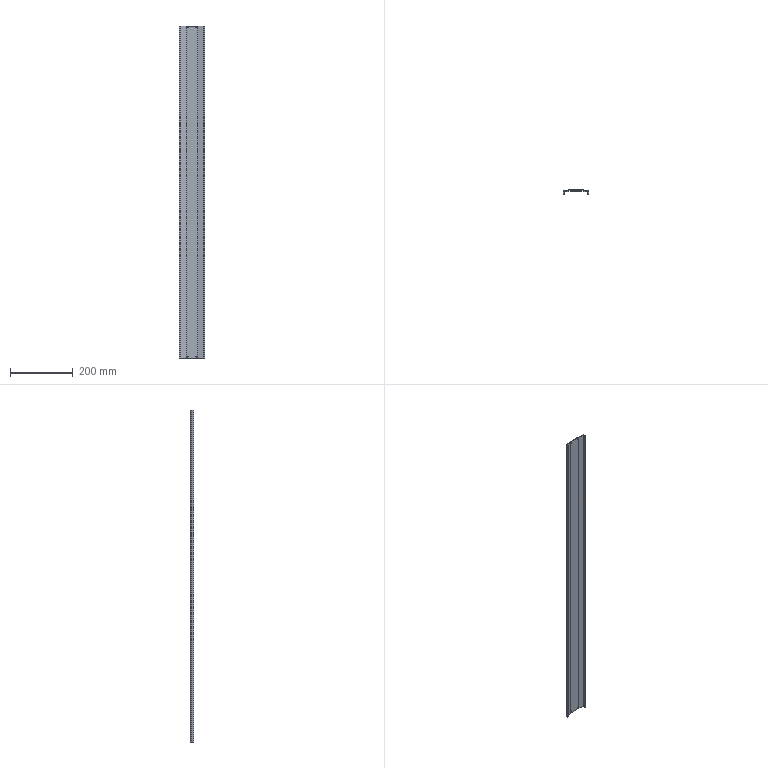Part | NX | 1 solid | 28 faces | box 82 x 11 x 1061 mm | volume 230950 mm3 | cylinder 14 | plane 14 | commonest cylinder face diameters 2 x6 4.5 x4 4 x2 10 x2
STEP:
#1=CARTESIAN_POINT('',(9079.118,2151.774,0.));
#2=VERTEX_POINT('',#1);
#3=CARTESIAN_POINT('',(9080.082,2150.506,0.));
#4=VERTEX_POINT('',#3);
#5=CARTESIAN_POINT('',(9080.082,2151.506,0.));
#6=DIRECTION('',(0.,0.,1.));
#7=DIRECTION('',(1.,0.,0.));
#8=AXIS2_PLACEMENT_3D('',#5,#6,#7);
#9=CIRCLE('',#8,1.);
#10=EDGE_CURVE('',#2,#4,#9,.T.);
#11=ORIENTED_EDGE('',*,*,#10,.T.);
#12=CARTESIAN_POINT('',(9080.082,2150.506,1061.));
#13=VERTEX_POINT('',#12);
#14=CARTESIAN_POINT('',(9080.082,2150.506,1061.));
#15=DIRECTION('',(0.,0.,-1.));
#16=VECTOR('',#15,1.);
#17=LINE('',#14,#16);
#18=EDGE_CURVE('',#13,#4,#17,.T.);
#19=ORIENTED_EDGE('',*,*,#18,.F.);
#20=CARTESIAN_POINT('',(9079.118,2151.774,1061.));
#21=VERTEX_POINT('',#20);
#22=CARTESIAN_POINT('',(9080.082,2151.506,1061.));
#23=DIRECTION('',(0.,0.,1.));
#24=DIRECTION('',(1.,0.,0.));
#25=AXIS2_PLACEMENT_3D('',#22,#23,#24);
#26=CIRCLE('',#25,1.);
#27=EDGE_CURVE('',#21,#13,#26,.T.);
#28=ORIENTED_EDGE('',*,*,#27,.F.);
#29=CARTESIAN_POINT('',(9079.118,2151.774,1061.));
#30=DIRECTION('',(0.,0.,-1.));
#31=VECTOR('',#30,1.);
#32=LINE('',#29,#31);
#33=EDGE_CURVE('',#21,#2,#32,.T.);
#34=ORIENTED_EDGE('',*,*,#33,.T.);
#35=EDGE_LOOP('',(#11,#19,#28,#34));
#36=FACE_OUTER_BOUND('',#35,.T.);
#37=CARTESIAN_POINT('',(9080.082,2151.506,1061.));
#38=DIRECTION('',(0.,0.,-1.));
#39=DIRECTION('',(1.,0.,0.));
#40=AXIS2_PLACEMENT_3D('',#37,#38,#39);
#41=CYLINDRICAL_SURFACE('',#40,1.);
#42=ADVANCED_FACE('',(#36),#41,.T.);
#43=CARTESIAN_POINT('',(9081.732,2150.506,0.));
#44=VERTEX_POINT('',#43);
#45=CARTESIAN_POINT('',(9080.082,2150.506,0.));
#46=DIRECTION('',(1.,0.,0.));
#47=VECTOR('',#46,1.);
#48=LINE('',#45,#47);
#49=EDGE_CURVE('',#4,#44,#48,.T.);
#50=ORIENTED_EDGE('',*,*,#49,.T.);
#51=CARTESIAN_POINT('',(9081.732,2150.506,1061.));
#52=VERTEX_POINT('',#51);
#53=CARTESIAN_POINT('',(9081.732,2150.506,1061.));
#54=DIRECTION('',(0.,0.,-1.));
#55=VECTOR('',#54,1.);
#56=LINE('',#53,#55);
#57=EDGE_CURVE('',#52,#44,#56,.T.);
#58=ORIENTED_EDGE('',*,*,#57,.F.);
#59=CARTESIAN_POINT('',(9080.082,2150.506,1061.));
#60=DIRECTION('',(1.,0.,0.));
#61=VECTOR('',#60,1.);
#62=LINE('',#59,#61);
#63=EDGE_CURVE('',#13,#52,#62,.T.);
#64=ORIENTED_EDGE('',*,*,#63,.F.);
#65=ORIENTED_EDGE('',*,*,#18,.T.);
#66=EDGE_LOOP('',(#50,#58,#64,#65));
#67=FACE_OUTER_BOUND('',#66,.T.);
#68=CARTESIAN_POINT('',(9080.082,2150.506,1061.));
#69=DIRECTION('',(0.,1.,0.));
#70=DIRECTION('',(0.,0.,-1.));
#71=AXIS2_PLACEMENT_3D('',#68,#69,#70);
#72=PLANE('',#71);
#73=ADVANCED_FACE('',(#67),#72,.F.);
#74=CARTESIAN_POINT('',(9082.732,2151.506,0.));
#75=VERTEX_POINT('',#74);
#76=CARTESIAN_POINT('',(9081.732,2151.506,0.));
#77=DIRECTION('',(0.,0.,1.));
#78=DIRECTION('',(1.,0.,0.));
#79=AXIS2_PLACEMENT_3D('',#76,#77,#78);
#80=CIRCLE('',#79,1.);
#81=EDGE_CURVE('',#44,#75,#80,.T.);
#82=ORIENTED_EDGE('',*,*,#81,.T.);
#83=CARTESIAN_POINT('',(9082.732,2151.506,1061.));
#84=VERTEX_POINT('',#83);
#85=CARTESIAN_POINT('',(9082.732,2151.506,1061.));
#86=DIRECTION('',(0.,0.,-1.));
#87=VECTOR('',#86,1.);
#88=LINE('',#85,#87);
#89=EDGE_CURVE('',#84,#75,#88,.T.);
#90=ORIENTED_EDGE('',*,*,#89,.F.);
#91=CARTESIAN_POINT('',(9081.732,2151.506,1061.));
#92=DIRECTION('',(0.,0.,1.));
#93=DIRECTION('',(1.,0.,0.));
#94=AXIS2_PLACEMENT_3D('',#91,#92,#93);
#95=CIRCLE('',#94,1.);
#96=EDGE_CURVE('',#52,#84,#95,.T.);
#97=ORIENTED_EDGE('',*,*,#96,.F.);
#98=ORIENTED_EDGE('',*,*,#57,.T.);
#99=EDGE_LOOP('',(#82,#90,#97,#98));
#100=FACE_OUTER_BOUND('',#99,.T.);
#101=CARTESIAN_POINT('',(9081.732,2151.506,1061.));
#102=DIRECTION('',(0.,0.,-1.));
#103=DIRECTION('',(1.,0.,0.));
#104=AXIS2_PLACEMENT_3D('',#101,#102,#103);
#105=CYLINDRICAL_SURFACE('',#104,1.);
#106=ADVANCED_FACE('',(#100),#105,.T.);
#107=CARTESIAN_POINT('',(9082.732,2155.69,0.));
#108=VERTEX_POINT('',#107);
#109=CARTESIAN_POINT('',(9082.732,2151.506,0.));
#110=DIRECTION('',(0.,1.,0.));
#111=VECTOR('',#110,1.);
#112=LINE('',#109,#111);
#113=EDGE_CURVE('',#75,#108,#112,.T.);
#114=ORIENTED_EDGE('',*,*,#113,.T.);
#115=CARTESIAN_POINT('',(9082.732,2155.69,1061.));
#116=VERTEX_POINT('',#115);
#117=CARTESIAN_POINT('',(9082.732,2155.69,1061.));
#118=DIRECTION('',(0.,0.,-1.));
#119=VECTOR('',#118,1.);
#120=LINE('',#117,#119);
#121=EDGE_CURVE('',#116,#108,#120,.T.);
#122=ORIENTED_EDGE('',*,*,#121,.F.);
#123=CARTESIAN_POINT('',(9082.732,2151.506,1061.));
#124=DIRECTION('',(0.,1.,0.));
#125=VECTOR('',#124,1.);
#126=LINE('',#123,#125);
#127=EDGE_CURVE('',#84,#116,#126,.T.);
#128=ORIENTED_EDGE('',*,*,#127,.F.);
#129=ORIENTED_EDGE('',*,*,#89,.T.);
#130=EDGE_LOOP('',(#114,#122,#128,#129));
#131=FACE_OUTER_BOUND('',#130,.T.);
#132=CARTESIAN_POINT('',(9082.732,2151.506,1061.));
#133=DIRECTION('',(-1.,0.,0.));
#134=DIRECTION('',(0.,0.,-1.));
#135=AXIS2_PLACEMENT_3D('',#132,#133,#134);
#136=PLANE('',#135);
#137=ADVANCED_FACE('',(#131),#136,.F.);
#138=CARTESIAN_POINT('',(9083.573,2156.677,0.));
#139=VERTEX_POINT('',#138);
#140=CARTESIAN_POINT('',(9083.732,2155.69,0.));
#141=DIRECTION('',(0.,0.,-1.));
#142=DIRECTION('',(1.,0.,0.));
#143=AXIS2_PLACEMENT_3D('',#140,#141,#142);
#144=CIRCLE('',#143,1.);
#145=EDGE_CURVE('',#108,#139,#144,.T.);
#146=ORIENTED_EDGE('',*,*,#145,.T.);
#147=CARTESIAN_POINT('',(9083.573,2156.677,1061.));
#148=VERTEX_POINT('',#147);
#149=CARTESIAN_POINT('',(9083.573,2156.677,1061.));
#150=DIRECTION('',(0.,0.,-1.));
#151=VECTOR('',#150,1.);
#152=LINE('',#149,#151);
#153=EDGE_CURVE('',#148,#139,#152,.T.);
#154=ORIENTED_EDGE('',*,*,#153,.F.);
#155=CARTESIAN_POINT('',(9083.732,2155.69,1061.));
#156=DIRECTION('',(0.,0.,-1.));
#157=DIRECTION('',(1.,0.,0.));
#158=AXIS2_PLACEMENT_3D('',#155,#156,#157);
#159=CIRCLE('',#158,1.);
#160=EDGE_CURVE('',#116,#148,#159,.T.);
#161=ORIENTED_EDGE('',*,*,#160,.F.);
#162=ORIENTED_EDGE('',*,*,#121,.T.);
#163=EDGE_LOOP('',(#146,#154,#161,#162));
#164=FACE_OUTER_BOUND('',#163,.T.);
#165=CARTESIAN_POINT('',(9083.732,2155.69,1061.));
#166=DIRECTION('',(0.,0.,-1.));
#167=DIRECTION('',(1.,0.,0.));
#168=AXIS2_PLACEMENT_3D('',#165,#166,#167);
#169=CYLINDRICAL_SURFACE('',#168,1.);
#170=ADVANCED_FACE('',(#164),#169,.F.);
#171=CARTESIAN_POINT('',(9101.149,2159.506,0.));
#172=VERTEX_POINT('',#171);
#173=CARTESIAN_POINT('',(9083.573,2156.677,0.));
#174=DIRECTION('',(0.9873,0.1589,0.));
#175=VECTOR('',#174,1.);
#176=LINE('',#173,#175);
#177=EDGE_CURVE('',#139,#172,#176,.T.);
#178=ORIENTED_EDGE('',*,*,#177,.T.);
#179=CARTESIAN_POINT('',(9101.149,2159.506,1061.));
#180=VERTEX_POINT('',#179);
#181=CARTESIAN_POINT('',(9101.149,2159.506,1061.));
#182=DIRECTION('',(0.,0.,-1.));
#183=VECTOR('',#182,1.);
#184=LINE('',#181,#183);
#185=EDGE_CURVE('',#180,#172,#184,.T.);
#186=ORIENTED_EDGE('',*,*,#185,.F.);
#187=CARTESIAN_POINT('',(9083.573,2156.677,1061.));
#188=DIRECTION('',(0.9873,0.1589,0.));
#189=VECTOR('',#188,1.);
#190=LINE('',#187,#189);
#191=EDGE_CURVE('',#148,#180,#190,.T.);
#192=ORIENTED_EDGE('',*,*,#191,.F.);
#193=ORIENTED_EDGE('',*,*,#153,.T.);
#194=EDGE_LOOP('',(#178,#186,#192,#193));
#195=FACE_OUTER_BOUND('',#194,.T.);
#196=CARTESIAN_POINT('',(9083.573,2156.677,1061.));
#197=DIRECTION('',(-0.1589,0.9873,0.));
#198=DIRECTION('',(0.9873,0.1589,0.));
#199=AXIS2_PLACEMENT_3D('',#196,#197,#198);
#200=PLANE('',#199);
#201=ADVANCED_FACE('',(#195),#200,.F.);
#202=CARTESIAN_POINT('',(9135.082,2159.506,1059.25));
#203=VERTEX_POINT('',#202);
#204=CARTESIAN_POINT('',(9135.082,2159.506,1057.));
#205=DIRECTION('',(0.,1.,0.));
#206=DIRECTION('',(0.,0.,1.));
#207=AXIS2_PLACEMENT_3D('',#204,#205,#206);
#208=CIRCLE('',#207,2.25);
#209=EDGE_CURVE('',#203,#203,#208,.T.);
#210=ORIENTED_EDGE('',*,*,#209,.T.);
#211=EDGE_LOOP('',(#210));
#212=FACE_BOUND('',#211,.T.);
#213=CARTESIAN_POINT('',(9135.082,2159.506,6.25));
#214=VERTEX_POINT('',#213);
#215=CARTESIAN_POINT('',(9135.082,2159.506,4.));
#216=DIRECTION('',(0.,1.,0.));
#217=DIRECTION('',(0.,0.,1.));
#218=AXIS2_PLACEMENT_3D('',#215,#216,#217);
#219=CIRCLE('',#218,2.25);
#220=EDGE_CURVE('',#214,#214,#219,.T.);
#221=ORIENTED_EDGE('',*,*,#220,.T.);
#222=EDGE_LOOP('',(#221));
#223=FACE_BOUND('',#222,.T.);
#224=CARTESIAN_POINT('',(9105.082,2159.506,1059.25));
#225=VERTEX_POINT('',#224);
#226=CARTESIAN_POINT('',(9105.082,2159.506,1057.));
#227=DIRECTION('',(0.,1.,0.));
#228=DIRECTION('',(0.,0.,1.));
#229=AXIS2_PLACEMENT_3D('',#226,#227,#228);
#230=CIRCLE('',#229,2.25);
#231=EDGE_CURVE('',#225,#225,#230,.T.);
#232=ORIENTED_EDGE('',*,*,#231,.T.);
#233=EDGE_LOOP('',(#232));
#234=FACE_BOUND('',#233,.T.);
#235=CARTESIAN_POINT('',(9105.082,2159.506,6.25));
#236=VERTEX_POINT('',#235);
#237=CARTESIAN_POINT('',(9105.082,2159.506,4.));
#238=DIRECTION('',(0.,1.,0.));
#239=DIRECTION('',(0.,0.,1.));
#240=AXIS2_PLACEMENT_3D('',#237,#238,#239);
#241=CIRCLE('',#240,2.25);
#242=EDGE_CURVE('',#236,#236,#241,.T.);
#243=ORIENTED_EDGE('',*,*,#242,.T.);
#244=EDGE_LOOP('',(#243));
#245=FACE_BOUND('',#244,.T.);
#246=CARTESIAN_POINT('',(9139.015,2159.506,0.));
#247=VERTEX_POINT('',#246);
#248=CARTESIAN_POINT('',(9101.149,2159.506,0.));
#249=DIRECTION('',(1.,0.,0.));
#250=VECTOR('',#249,1.);
#251=LINE('',#248,#250);
#252=EDGE_CURVE('',#172,#247,#251,.T.);
#253=ORIENTED_EDGE('',*,*,#252,.T.);
#254=CARTESIAN_POINT('',(9139.015,2159.506,1061.));
#255=VERTEX_POINT('',#254);
#256=CARTESIAN_POINT('',(9139.015,2159.506,1061.));
#257=DIRECTION('',(0.,0.,-1.));
#258=VECTOR('',#257,1.);
#259=LINE('',#256,#258);
#260=EDGE_CURVE('',#255,#247,#259,.T.);
#261=ORIENTED_EDGE('',*,*,#260,.F.);
#262=CARTESIAN_POINT('',(9101.149,2159.506,1061.));
#263=DIRECTION('',(1.,0.,0.));
#264=VECTOR('',#263,1.);
#265=LINE('',#262,#264);
#266=EDGE_CURVE('',#180,#255,#265,.T.);
#267=ORIENTED_EDGE('',*,*,#266,.F.);
#268=ORIENTED_EDGE('',*,*,#185,.T.);
#269=EDGE_LOOP('',(#253,#261,#267,#268));
#270=FACE_BOUND('',#269,.T.);
#271=CARTESIAN_POINT('',(9101.149,2159.506,1061.));
#272=DIRECTION('',(0.,1.,0.));
#273=DIRECTION('',(0.,0.,-1.));
#274=AXIS2_PLACEMENT_3D('',#271,#272,#273);
#275=PLANE('',#274);
#276=ADVANCED_FACE('',(#212,#223,#234,#245,#270),#275,.F.);
#277=CARTESIAN_POINT('',(9156.591,2156.677,0.));
#278=VERTEX_POINT('',#277);
#279=CARTESIAN_POINT('',(9139.015,2159.506,0.));
#280=DIRECTION('',(0.9873,-0.1589,0.));
#281=VECTOR('',#280,1.);
#282=LINE('',#279,#281);
#283=EDGE_CURVE('',#247,#278,#282,.T.);
#284=ORIENTED_EDGE('',*,*,#283,.T.);
#285=CARTESIAN_POINT('',(9156.591,2156.677,1061.));
#286=VERTEX_POINT('',#285);
#287=CARTESIAN_POINT('',(9156.591,2156.677,1061.));
#288=DIRECTION('',(0.,0.,-1.));
#289=VECTOR('',#288,1.);
#290=LINE('',#287,#289);
#291=EDGE_CURVE('',#286,#278,#290,.T.);
#292=ORIENTED_EDGE('',*,*,#291,.F.);
#293=CARTESIAN_POINT('',(9139.015,2159.506,1061.));
#294=DIRECTION('',(0.9873,-0.1589,0.));
#295=VECTOR('',#294,1.);
#296=LINE('',#293,#295);
#297=EDGE_CURVE('',#255,#286,#296,.T.);
#298=ORIENTED_EDGE('',*,*,#297,.F.);
#299=ORIENTED_EDGE('',*,*,#260,.T.);
#300=EDGE_LOOP('',(#284,#292,#298,#299));
#301=FACE_OUTER_BOUND('',#300,.T.);
#302=CARTESIAN_POINT('',(9139.015,2159.506,1061.));
#303=DIRECTION('',(0.1589,0.9873,0.));
#304=DIRECTION('',(0.9873,-0.1589,0.));
#305=AXIS2_PLACEMENT_3D('',#302,#303,#304);
#306=PLANE('',#305);
#307=ADVANCED_FACE('',(#301),#306,.F.);
#308=CARTESIAN_POINT('',(9157.432,2155.69,0.));
#309=VERTEX_POINT('',#308);
#310=CARTESIAN_POINT('',(9156.432,2155.69,0.));
#311=DIRECTION('',(0.,0.,-1.));
#312=DIRECTION('',(1.,0.,0.));
#313=AXIS2_PLACEMENT_3D('',#310,#311,#312);
#314=CIRCLE('',#313,1.);
#315=EDGE_CURVE('',#278,#309,#314,.T.);
#316=ORIENTED_EDGE('',*,*,#315,.T.);
#317=CARTESIAN_POINT('',(9157.432,2155.69,1061.));
#318=VERTEX_POINT('',#317);
#319=CARTESIAN_POINT('',(9157.432,2155.69,1061.));
#320=DIRECTION('',(0.,0.,-1.));
#321=VECTOR('',#320,1.);
#322=LINE('',#319,#321);
#323=EDGE_CURVE('',#318,#309,#322,.T.);
#324=ORIENTED_EDGE('',*,*,#323,.F.);
#325=CARTESIAN_POINT('',(9156.432,2155.69,1061.));
#326=DIRECTION('',(0.,0.,-1.));
#327=DIRECTION('',(1.,0.,0.));
#328=AXIS2_PLACEMENT_3D('',#325,#326,#327);
#329=CIRCLE('',#328,1.);
#330=EDGE_CURVE('',#286,#318,#329,.T.);
#331=ORIENTED_EDGE('',*,*,#330,.F.);
#332=ORIENTED_EDGE('',*,*,#291,.T.);
#333=EDGE_LOOP('',(#316,#324,#331,#332));
#334=FACE_OUTER_BOUND('',#333,.T.);
#335=CARTESIAN_POINT('',(9156.432,2155.69,1061.));
#336=DIRECTION('',(0.,0.,-1.));
#337=DIRECTION('',(1.,0.,0.));
#338=AXIS2_PLACEMENT_3D('',#335,#336,#337);
#339=CYLINDRICAL_SURFACE('',#338,1.);
#340=ADVANCED_FACE('',(#334),#339,.F.);
#341=CARTESIAN_POINT('',(9157.432,2151.506,0.));
#342=VERTEX_POINT('',#341);
#343=CARTESIAN_POINT('',(9157.432,2155.69,0.));
#344=DIRECTION('',(0.,-1.,0.));
#345=VECTOR('',#344,1.);
#346=LINE('',#343,#345);
#347=EDGE_CURVE('',#309,#342,#346,.T.);
#348=ORIENTED_EDGE('',*,*,#347,.T.);
#349=CARTESIAN_POINT('',(9157.432,2151.506,1061.));
#350=VERTEX_POINT('',#349);
#351=CARTESIAN_POINT('',(9157.432,2151.506,1061.));
#352=DIRECTION('',(0.,0.,-1.));
#353=VECTOR('',#352,1.);
#354=LINE('',#351,#353);
#355=EDGE_CURVE('',#350,#342,#354,.T.);
#356=ORIENTED_EDGE('',*,*,#355,.F.);
#357=CARTESIAN_POINT('',(9157.432,2155.69,1061.));
#358=DIRECTION('',(0.,-1.,0.));
#359=VECTOR('',#358,1.);
#360=LINE('',#357,#359);
#361=EDGE_CURVE('',#318,#350,#360,.T.);
#362=ORIENTED_EDGE('',*,*,#361,.F.);
#363=ORIENTED_EDGE('',*,*,#323,.T.);
#364=EDGE_LOOP('',(#348,#356,#362,#363));
#365=FACE_OUTER_BOUND('',#364,.T.);
#366=CARTESIAN_POINT('',(9157.432,2155.69,1061.));
#367=DIRECTION('',(1.,0.,0.));
#368=DIRECTION('',(0.,0.,1.));
#369=AXIS2_PLACEMENT_3D('',#366,#367,#368);
#370=PLANE('',#369);
#371=ADVANCED_FACE('',(#365),#370,.F.);
#372=CARTESIAN_POINT('',(9158.432,2150.506,0.));
#373=VERTEX_POINT('',#372);
#374=CARTESIAN_POINT('',(9158.432,2151.506,0.));
#375=DIRECTION('',(0.,0.,1.));
#376=DIRECTION('',(1.,0.,0.));
#377=AXIS2_PLACEMENT_3D('',#374,#375,#376);
#378=CIRCLE('',#377,1.);
#379=EDGE_CURVE('',#342,#373,#378,.T.);
#380=ORIENTED_EDGE('',*,*,#379,.T.);
#381=CARTESIAN_POINT('',(9158.432,2150.506,1061.));
#382=VERTEX_POINT('',#381);
#383=CARTESIAN_POINT('',(9158.432,2150.506,1061.));
#384=DIRECTION('',(0.,0.,-1.));
#385=VECTOR('',#384,1.);
#386=LINE('',#383,#385);
#387=EDGE_CURVE('',#382,#373,#386,.T.);
#388=ORIENTED_EDGE('',*,*,#387,.F.);
#389=CARTESIAN_POINT('',(9158.432,2151.506,1061.));
#390=DIRECTION('',(0.,0.,1.));
#391=DIRECTION('',(1.,0.,0.));
#392=AXIS2_PLACEMENT_3D('',#389,#390,#391);
#393=CIRCLE('',#392,1.);
#394=EDGE_CURVE('',#350,#382,#393,.T.);
#395=ORIENTED_EDGE('',*,*,#394,.F.);
#396=ORIENTED_EDGE('',*,*,#355,.T.);
#397=EDGE_LOOP('',(#380,#388,#395,#396));
#398=FACE_OUTER_BOUND('',#397,.T.);
#399=CARTESIAN_POINT('',(9158.432,2151.506,1061.));
#400=DIRECTION('',(0.,0.,-1.));
#401=DIRECTION('',(1.,0.,0.));
#402=AXIS2_PLACEMENT_3D('',#399,#400,#401);
#403=CYLINDRICAL_SURFACE('',#402,1.);
#404=ADVANCED_FACE('',(#398),#403,.T.);
#405=CARTESIAN_POINT('',(9160.082,2150.506,0.));
#406=VERTEX_POINT('',#405);
#407=CARTESIAN_POINT('',(9158.432,2150.506,0.));
#408=DIRECTION('',(1.,0.,0.));
#409=VECTOR('',#408,1.);
#410=LINE('',#407,#409);
#411=EDGE_CURVE('',#373,#406,#410,.T.);
#412=ORIENTED_EDGE('',*,*,#411,.T.);
#413=CARTESIAN_POINT('',(9160.082,2150.506,1061.));
#414=VERTEX_POINT('',#413);
#415=CARTESIAN_POINT('',(9160.082,2150.506,1061.));
#416=DIRECTION('',(0.,0.,-1.));
#417=VECTOR('',#416,1.);
#418=LINE('',#415,#417);
#419=EDGE_CURVE('',#414,#406,#418,.T.);
#420=ORIENTED_EDGE('',*,*,#419,.F.);
#421=CARTESIAN_POINT('',(9158.432,2150.506,1061.));
#422=DIRECTION('',(1.,0.,0.));
#423=VECTOR('',#422,1.);
#424=LINE('',#421,#423);
#425=EDGE_CURVE('',#382,#414,#424,.T.);
#426=ORIENTED_EDGE('',*,*,#425,.F.);
#427=ORIENTED_EDGE('',*,*,#387,.T.);
#428=EDGE_LOOP('',(#412,#420,#426,#427));
#429=FACE_OUTER_BOUND('',#428,.T.);
#430=CARTESIAN_POINT('',(9158.432,2150.506,1061.));
#431=DIRECTION('',(0.,1.,0.));
#432=DIRECTION('',(0.,0.,-1.));
#433=AXIS2_PLACEMENT_3D('',#430,#431,#432);
#434=PLANE('',#433);
#435=ADVANCED_FACE('',(#429),#434,.F.);
#436=CARTESIAN_POINT('',(9161.045,2151.774,0.));
#437=VERTEX_POINT('',#436);
#438=CARTESIAN_POINT('',(9160.082,2151.506,0.));
#439=DIRECTION('',(0.,0.,1.));
#440=DIRECTION('',(1.,0.,0.));
#441=AXIS2_PLACEMENT_3D('',#438,#439,#440);
#442=CIRCLE('',#441,1.);
#443=EDGE_CURVE('',#406,#437,#442,.T.);
#444=ORIENTED_EDGE('',*,*,#443,.T.);
#445=CARTESIAN_POINT('',(9161.045,2151.774,1061.));
#446=VERTEX_POINT('',#445);
#447=CARTESIAN_POINT('',(9161.045,2151.774,1061.));
#448=DIRECTION('',(0.,0.,-1.));
#449=VECTOR('',#448,1.);
#450=LINE('',#447,#449);
#451=EDGE_CURVE('',#446,#437,#450,.T.);
#452=ORIENTED_EDGE('',*,*,#451,.F.);
#453=CARTESIAN_POINT('',(9160.082,2151.506,1061.));
#454=DIRECTION('',(0.,0.,1.));
#455=DIRECTION('',(1.,0.,0.));
#456=AXIS2_PLACEMENT_3D('',#453,#454,#455);
#457=CIRCLE('',#456,1.);
#458=EDGE_CURVE('',#414,#446,#457,.T.);
#459=ORIENTED_EDGE('',*,*,#458,.F.);
#460=ORIENTED_EDGE('',*,*,#419,.T.);
#461=EDGE_LOOP('',(#444,#452,#459,#460));
#462=FACE_OUTER_BOUND('',#461,.T.);
#463=CARTESIAN_POINT('',(9160.082,2151.506,1061.));
#464=DIRECTION('',(0.,0.,-1.));
#465=DIRECTION('',(1.,0.,0.));
#466=AXIS2_PLACEMENT_3D('',#463,#464,#465);
#467=CYLINDRICAL_SURFACE('',#466,1.);
#468=ADVANCED_FACE('',(#462),#467,.T.);
#469=CARTESIAN_POINT('',(9159.359,2157.842,0.));
#470=VERTEX_POINT('',#469);
#471=CARTESIAN_POINT('',(9161.045,2151.774,0.));
#472=DIRECTION('',(-0.2678,0.9635,0.));
#473=VECTOR('',#472,1.);
#474=LINE('',#471,#473);
#475=EDGE_CURVE('',#437,#470,#474,.T.);
#476=ORIENTED_EDGE('',*,*,#475,.T.);
#477=CARTESIAN_POINT('',(9159.359,2157.842,1061.));
#478=VERTEX_POINT('',#477);
#479=CARTESIAN_POINT('',(9159.359,2157.842,1061.));
#480=DIRECTION('',(0.,0.,-1.));
#481=VECTOR('',#480,1.);
#482=LINE('',#479,#481);
#483=EDGE_CURVE('',#478,#470,#482,.T.);
#484=ORIENTED_EDGE('',*,*,#483,.F.);
#485=CARTESIAN_POINT('',(9161.045,2151.774,1061.));
#486=DIRECTION('',(-0.2678,0.9635,0.));
#487=VECTOR('',#486,1.);
#488=LINE('',#485,#487);
#489=EDGE_CURVE('',#446,#478,#488,.T.);
#490=ORIENTED_EDGE('',*,*,#489,.F.);
#491=ORIENTED_EDGE('',*,*,#451,.T.);
#492=EDGE_LOOP('',(#476,#484,#490,#491));
#493=FACE_OUTER_BOUND('',#492,.T.);
#494=CARTESIAN_POINT('',(9161.045,2151.774,1061.));
#495=DIRECTION('',(-0.9635,-0.2678,0.));
#496=DIRECTION('',(-0.2678,0.9635,0.));
#497=AXIS2_PLACEMENT_3D('',#494,#495,#496);
#498=PLANE('',#497);
#499=ADVANCED_FACE('',(#493),#498,.F.);
#500=CARTESIAN_POINT('',(9157.719,2159.285,0.));
#501=VERTEX_POINT('',#500);
#502=CARTESIAN_POINT('',(9157.432,2157.306,0.));
#503=DIRECTION('',(0.,0.,1.));
#504=DIRECTION('',(1.,0.,0.));
#505=AXIS2_PLACEMENT_3D('',#502,#503,#504);
#506=CIRCLE('',#505,2.);
#507=EDGE_CURVE('',#470,#501,#506,.T.);
#508=ORIENTED_EDGE('',*,*,#507,.T.);
#509=CARTESIAN_POINT('',(9157.719,2159.285,1061.));
#510=VERTEX_POINT('',#509);
#511=CARTESIAN_POINT('',(9157.719,2159.285,1061.));
#512=DIRECTION('',(0.,0.,-1.));
#513=VECTOR('',#512,1.);
#514=LINE('',#511,#513);
#515=EDGE_CURVE('',#510,#501,#514,.T.);
#516=ORIENTED_EDGE('',*,*,#515,.F.);
#517=CARTESIAN_POINT('',(9157.432,2157.306,1061.));
#518=DIRECTION('',(0.,0.,1.));
#519=DIRECTION('',(1.,0.,0.));
#520=AXIS2_PLACEMENT_3D('',#517,#518,#519);
#521=CIRCLE('',#520,2.);
#522=EDGE_CURVE('',#478,#510,#521,.T.);
#523=ORIENTED_EDGE('',*,*,#522,.F.);
#524=ORIENTED_EDGE('',*,*,#483,.T.);
#525=EDGE_LOOP('',(#508,#516,#523,#524));
#526=FACE_OUTER_BOUND('',#525,.T.);
#527=CARTESIAN_POINT('',(9157.432,2157.306,1061.));
#528=DIRECTION('',(0.,0.,-1.));
#529=DIRECTION('',(1.,0.,0.));
#530=AXIS2_PLACEMENT_3D('',#527,#528,#529);
#531=CYLINDRICAL_SURFACE('',#530,2.);
#532=ADVANCED_FACE('',(#526),#531,.T.);
#533=CARTESIAN_POINT('',(9142.801,2161.454,0.));
#534=VERTEX_POINT('',#533);
#535=CARTESIAN_POINT('',(9157.719,2159.285,0.));
#536=DIRECTION('',(-0.9896,0.1439,0.));
#537=VECTOR('',#536,1.);
#538=LINE('',#535,#537);
#539=EDGE_CURVE('',#501,#534,#538,.T.);
#540=ORIENTED_EDGE('',*,*,#539,.T.);
#541=CARTESIAN_POINT('',(9142.801,2161.454,1061.));
#542=VERTEX_POINT('',#541);
#543=CARTESIAN_POINT('',(9142.801,2161.454,1061.));
#544=DIRECTION('',(0.,0.,-1.));
#545=VECTOR('',#544,1.);
#546=LINE('',#543,#545);
#547=EDGE_CURVE('',#542,#534,#546,.T.);
#548=ORIENTED_EDGE('',*,*,#547,.F.);
#549=CARTESIAN_POINT('',(9157.719,2159.285,1061.));
#550=DIRECTION('',(-0.9896,0.1439,0.));
#551=VECTOR('',#550,1.);
#552=LINE('',#549,#551);
#553=EDGE_CURVE('',#510,#542,#552,.T.);
#554=ORIENTED_EDGE('',*,*,#553,.F.);
#555=ORIENTED_EDGE('',*,*,#515,.T.);
#556=EDGE_LOOP('',(#540,#548,#554,#555));
#557=FACE_OUTER_BOUND('',#556,.T.);
#558=CARTESIAN_POINT('',(9157.719,2159.285,1061.));
#559=DIRECTION('',(-0.1439,-0.9896,0.));
#560=DIRECTION('',(-0.9896,0.1439,0.));
#561=AXIS2_PLACEMENT_3D('',#558,#559,#560);
#562=PLANE('',#561);
#563=ADVANCED_FACE('',(#557),#562,.F.);
#564=CARTESIAN_POINT('',(9142.082,2161.506,0.));
#565=VERTEX_POINT('',#564);
#566=CARTESIAN_POINT('',(9142.082,2156.506,0.));
#567=DIRECTION('',(0.,0.,1.));
#568=DIRECTION('',(1.,0.,0.));
#569=AXIS2_PLACEMENT_3D('',#566,#567,#568);
#570=CIRCLE('',#569,5.);
#571=EDGE_CURVE('',#534,#565,#570,.T.);
#572=ORIENTED_EDGE('',*,*,#571,.T.);
#573=CARTESIAN_POINT('',(9142.082,2161.506,1061.));
#574=VERTEX_POINT('',#573);
#575=CARTESIAN_POINT('',(9142.082,2161.506,1061.));
#576=DIRECTION('',(0.,0.,-1.));
#577=VECTOR('',#576,1.);
#578=LINE('',#575,#577);
#579=EDGE_CURVE('',#574,#565,#578,.T.);
#580=ORIENTED_EDGE('',*,*,#579,.F.);
#581=CARTESIAN_POINT('',(9142.082,2156.506,1061.));
#582=DIRECTION('',(0.,0.,1.));
#583=DIRECTION('',(1.,0.,0.));
#584=AXIS2_PLACEMENT_3D('',#581,#582,#583);
#585=CIRCLE('',#584,5.);
#586=EDGE_CURVE('',#542,#574,#585,.T.);
#587=ORIENTED_EDGE('',*,*,#586,.F.);
#588=ORIENTED_EDGE('',*,*,#547,.T.);
#589=EDGE_LOOP('',(#572,#580,#587,#588));
#590=FACE_OUTER_BOUND('',#589,.T.);
#591=CARTESIAN_POINT('',(9142.082,2156.506,1061.));
#592=DIRECTION('',(0.,0.,-1.));
#593=DIRECTION('',(1.,0.,0.));
#594=AXIS2_PLACEMENT_3D('',#591,#592,#593);
#595=CYLINDRICAL_SURFACE('',#594,5.);
#596=ADVANCED_FACE('',(#590),#595,.T.);
#597=CARTESIAN_POINT('',(9135.082,2161.506,1054.75));
#598=VERTEX_POINT('',#597);
#599=CARTESIAN_POINT('',(9135.082,2161.506,1057.));
#600=DIRECTION('',(0.,-1.,0.));
#601=DIRECTION('',(0.,0.,-1.));
#602=AXIS2_PLACEMENT_3D('',#599,#600,#601);
#603=CIRCLE('',#602,2.25);
#604=EDGE_CURVE('',#598,#598,#603,.T.);
#605=ORIENTED_EDGE('',*,*,#604,.T.);
#606=EDGE_LOOP('',(#605));
#607=FACE_BOUND('',#606,.T.);
#608=CARTESIAN_POINT('',(9135.082,2161.506,1.75));
#609=VERTEX_POINT('',#608);
#610=CARTESIAN_POINT('',(9135.082,2161.506,4.));
#611=DIRECTION('',(0.,-1.,0.));
#612=DIRECTION('',(0.,0.,-1.));
#613=AXIS2_PLACEMENT_3D('',#610,#611,#612);
#614=CIRCLE('',#613,2.25);
#615=EDGE_CURVE('',#609,#609,#614,.T.);
#616=ORIENTED_EDGE('',*,*,#615,.T.);
#617=EDGE_LOOP('',(#616));
#618=FACE_BOUND('',#617,.T.);
#619=CARTESIAN_POINT('',(9105.082,2161.506,1054.75));
#620=VERTEX_POINT('',#619);
#621=CARTESIAN_POINT('',(9105.082,2161.506,1057.));
#622=DIRECTION('',(0.,-1.,0.));
#623=DIRECTION('',(0.,0.,-1.));
#624=AXIS2_PLACEMENT_3D('',#621,#622,#623);
#625=CIRCLE('',#624,2.25);
#626=EDGE_CURVE('',#620,#620,#625,.T.);
#627=ORIENTED_EDGE('',*,*,#626,.T.);
#628=EDGE_LOOP('',(#627));
#629=FACE_BOUND('',#628,.T.);
#630=CARTESIAN_POINT('',(9105.082,2161.506,1.75));
#631=VERTEX_POINT('',#630);
#632=CARTESIAN_POINT('',(9105.082,2161.506,4.));
#633=DIRECTION('',(0.,-1.,0.));
#634=DIRECTION('',(0.,0.,-1.));
#635=AXIS2_PLACEMENT_3D('',#632,#633,#634);
#636=CIRCLE('',#635,2.25);
#637=EDGE_CURVE('',#631,#631,#636,.T.);
#638=ORIENTED_EDGE('',*,*,#637,.T.);
#639=EDGE_LOOP('',(#638));
#640=FACE_BOUND('',#639,.T.);
#641=CARTESIAN_POINT('',(9098.082,2161.506,0.));
#642=VERTEX_POINT('',#641);
#643=CARTESIAN_POINT('',(9142.082,2161.506,0.));
#644=DIRECTION('',(-1.,0.,0.));
#645=VECTOR('',#644,1.);
#646=LINE('',#643,#645);
#647=EDGE_CURVE('',#565,#642,#646,.T.);
#648=ORIENTED_EDGE('',*,*,#647,.T.);
#649=CARTESIAN_POINT('',(9098.082,2161.506,1061.));
#650=VERTEX_POINT('',#649);
#651=CARTESIAN_POINT('',(9098.082,2161.506,1061.));
#652=DIRECTION('',(0.,0.,-1.));
#653=VECTOR('',#652,1.);
#654=LINE('',#651,#653);
#655=EDGE_CURVE('',#650,#642,#654,.T.);
#656=ORIENTED_EDGE('',*,*,#655,.F.);
#657=CARTESIAN_POINT('',(9142.082,2161.506,1061.));
#658=DIRECTION('',(-1.,0.,0.));
#659=VECTOR('',#658,1.);
#660=LINE('',#657,#659);
#661=EDGE_CURVE('',#574,#650,#660,.T.);
#662=ORIENTED_EDGE('',*,*,#661,.F.);
#663=ORIENTED_EDGE('',*,*,#579,.T.);
#664=EDGE_LOOP('',(#648,#656,#662,#663));
#665=FACE_BOUND('',#664,.T.);
#666=CARTESIAN_POINT('',(9142.082,2161.506,1061.));
#667=DIRECTION('',(0.,-1.,0.));
#668=DIRECTION('',(0.,0.,1.));
#669=AXIS2_PLACEMENT_3D('',#666,#667,#668);
#670=PLANE('',#669);
#671=ADVANCED_FACE('',(#607,#618,#629,#640,#665),#670,.F.);
#672=CARTESIAN_POINT('',(9097.362,2161.454,0.));
#673=VERTEX_POINT('',#672);
#674=CARTESIAN_POINT('',(9098.082,2156.506,0.));
#675=DIRECTION('',(0.,0.,1.));
#676=DIRECTION('',(1.,0.,0.));
#677=AXIS2_PLACEMENT_3D('',#674,#675,#676);
#678=CIRCLE('',#677,5.);
#679=EDGE_CURVE('',#642,#673,#678,.T.);
#680=ORIENTED_EDGE('',*,*,#679,.T.);
#681=CARTESIAN_POINT('',(9097.362,2161.454,1061.));
#682=VERTEX_POINT('',#681);
#683=CARTESIAN_POINT('',(9097.362,2161.454,1061.));
#684=DIRECTION('',(0.,0.,-1.));
#685=VECTOR('',#684,1.);
#686=LINE('',#683,#685);
#687=EDGE_CURVE('',#682,#673,#686,.T.);
#688=ORIENTED_EDGE('',*,*,#687,.F.);
#689=CARTESIAN_POINT('',(9098.082,2156.506,1061.));
#690=DIRECTION('',(0.,0.,1.));
#691=DIRECTION('',(1.,0.,0.));
#692=AXIS2_PLACEMENT_3D('',#689,#690,#691);
#693=CIRCLE('',#692,5.);
#694=EDGE_CURVE('',#650,#682,#693,.T.);
#695=ORIENTED_EDGE('',*,*,#694,.F.);
#696=ORIENTED_EDGE('',*,*,#655,.T.);
#697=EDGE_LOOP('',(#680,#688,#695,#696));
#698=FACE_OUTER_BOUND('',#697,.T.);
#699=CARTESIAN_POINT('',(9098.082,2156.506,1061.));
#700=DIRECTION('',(0.,0.,-1.));
#701=DIRECTION('',(1.,0.,0.));
#702=AXIS2_PLACEMENT_3D('',#699,#700,#701);
#703=CYLINDRICAL_SURFACE('',#702,5.);
#704=ADVANCED_FACE('',(#698),#703,.T.);
#705=CARTESIAN_POINT('',(9082.444,2159.285,0.));
#706=VERTEX_POINT('',#705);
#707=CARTESIAN_POINT('',(9097.362,2161.454,0.));
#708=DIRECTION('',(-0.9896,-0.1439,0.));
#709=VECTOR('',#708,1.);
#710=LINE('',#707,#709);
#711=EDGE_CURVE('',#673,#706,#710,.T.);
#712=ORIENTED_EDGE('',*,*,#711,.T.);
#713=CARTESIAN_POINT('',(9082.444,2159.285,1061.));
#714=VERTEX_POINT('',#713);
#715=CARTESIAN_POINT('',(9082.444,2159.285,1061.));
#716=DIRECTION('',(0.,0.,-1.));
#717=VECTOR('',#716,1.);
#718=LINE('',#715,#717);
#719=EDGE_CURVE('',#714,#706,#718,.T.);
#720=ORIENTED_EDGE('',*,*,#719,.F.);
#721=CARTESIAN_POINT('',(9097.362,2161.454,1061.));
#722=DIRECTION('',(-0.9896,-0.1439,0.));
#723=VECTOR('',#722,1.);
#724=LINE('',#721,#723);
#725=EDGE_CURVE('',#682,#714,#724,.T.);
#726=ORIENTED_EDGE('',*,*,#725,.F.);
#727=ORIENTED_EDGE('',*,*,#687,.T.);
#728=EDGE_LOOP('',(#712,#720,#726,#727));
#729=FACE_OUTER_BOUND('',#728,.T.);
#730=CARTESIAN_POINT('',(9097.362,2161.454,1061.));
#731=DIRECTION('',(0.1439,-0.9896,0.));
#732=DIRECTION('',(-0.9896,-0.1439,0.));
#733=AXIS2_PLACEMENT_3D('',#730,#731,#732);
#734=PLANE('',#733);
#735=ADVANCED_FACE('',(#729),#734,.F.);
#736=CARTESIAN_POINT('',(9080.805,2157.842,0.));
#737=VERTEX_POINT('',#736);
#738=CARTESIAN_POINT('',(9082.732,2157.306,0.));
#739=DIRECTION('',(0.,0.,1.));
#740=DIRECTION('',(1.,0.,0.));
#741=AXIS2_PLACEMENT_3D('',#738,#739,#740);
#742=CIRCLE('',#741,2.);
#743=EDGE_CURVE('',#706,#737,#742,.T.);
#744=ORIENTED_EDGE('',*,*,#743,.T.);
#745=CARTESIAN_POINT('',(9080.805,2157.842,1061.));
#746=VERTEX_POINT('',#745);
#747=CARTESIAN_POINT('',(9080.805,2157.842,1061.));
#748=DIRECTION('',(0.,0.,-1.));
#749=VECTOR('',#748,1.);
#750=LINE('',#747,#749);
#751=EDGE_CURVE('',#746,#737,#750,.T.);
#752=ORIENTED_EDGE('',*,*,#751,.F.);
#753=CARTESIAN_POINT('',(9082.732,2157.306,1061.));
#754=DIRECTION('',(0.,0.,1.));
#755=DIRECTION('',(1.,0.,0.));
#756=AXIS2_PLACEMENT_3D('',#753,#754,#755);
#757=CIRCLE('',#756,2.);
#758=EDGE_CURVE('',#714,#746,#757,.T.);
#759=ORIENTED_EDGE('',*,*,#758,.F.);
#760=ORIENTED_EDGE('',*,*,#719,.T.);
#761=EDGE_LOOP('',(#744,#752,#759,#760));
#762=FACE_OUTER_BOUND('',#761,.T.);
#763=CARTESIAN_POINT('',(9082.732,2157.306,1061.));
#764=DIRECTION('',(0.,0.,-1.));
#765=DIRECTION('',(1.,0.,0.));
#766=AXIS2_PLACEMENT_3D('',#763,#764,#765);
#767=CYLINDRICAL_SURFACE('',#766,2.);
#768=ADVANCED_FACE('',(#762),#767,.T.);
#769=CARTESIAN_POINT('',(9080.805,2157.842,0.));
#770=DIRECTION('',(-0.2678,-0.9635,0.));
#771=VECTOR('',#770,1.);
#772=LINE('',#769,#771);
#773=EDGE_CURVE('',#737,#2,#772,.T.);
#774=ORIENTED_EDGE('',*,*,#773,.T.);
#775=ORIENTED_EDGE('',*,*,#33,.F.);
#776=CARTESIAN_POINT('',(9080.805,2157.842,1061.));
#777=DIRECTION('',(-0.2678,-0.9635,0.));
#778=VECTOR('',#777,1.);
#779=LINE('',#776,#778);
#780=EDGE_CURVE('',#746,#21,#779,.T.);
#781=ORIENTED_EDGE('',*,*,#780,.F.);
#782=ORIENTED_EDGE('',*,*,#751,.T.);
#783=EDGE_LOOP('',(#774,#775,#781,#782));
#784=FACE_OUTER_BOUND('',#783,.T.);
#785=CARTESIAN_POINT('',(9080.805,2157.842,1061.));
#786=DIRECTION('',(0.9635,-0.2678,0.));
#787=DIRECTION('',(-0.2678,-0.9635,0.));
#788=AXIS2_PLACEMENT_3D('',#785,#786,#787);
#789=PLANE('',#788);
#790=ADVANCED_FACE('',(#784),#789,.F.);
#791=ORIENTED_EDGE('',*,*,#27,.T.);
#792=ORIENTED_EDGE('',*,*,#63,.T.);
#793=ORIENTED_EDGE('',*,*,#96,.T.);
#794=ORIENTED_EDGE('',*,*,#127,.T.);
#795=ORIENTED_EDGE('',*,*,#160,.T.);
#796=ORIENTED_EDGE('',*,*,#191,.T.);
#797=ORIENTED_EDGE('',*,*,#266,.T.);
#798=ORIENTED_EDGE('',*,*,#297,.T.);
#799=ORIENTED_EDGE('',*,*,#330,.T.);
#800=ORIENTED_EDGE('',*,*,#361,.T.);
#801=ORIENTED_EDGE('',*,*,#394,.T.);
#802=ORIENTED_EDGE('',*,*,#425,.T.);
#803=ORIENTED_EDGE('',*,*,#458,.T.);
#804=ORIENTED_EDGE('',*,*,#489,.T.);
#805=ORIENTED_EDGE('',*,*,#522,.T.);
#806=ORIENTED_EDGE('',*,*,#553,.T.);
#807=ORIENTED_EDGE('',*,*,#586,.T.);
#808=ORIENTED_EDGE('',*,*,#661,.T.);
#809=ORIENTED_EDGE('',*,*,#694,.T.);
#810=ORIENTED_EDGE('',*,*,#725,.T.);
#811=ORIENTED_EDGE('',*,*,#758,.T.);
#812=ORIENTED_EDGE('',*,*,#780,.T.);
#813=EDGE_LOOP('',(#791,#792,#793,#794,#795,#796,#797,#798,#799,#800,#801,#802,#803,#804,#805,#806,#807,#808,#809,#810,#811,#812));
#814=FACE_OUTER_BOUND('',#813,.T.);
#815=CARTESIAN_POINT('',(9080.082,2151.506,1061.));
#816=DIRECTION('',(0.,0.,1.));
#817=DIRECTION('',(-1.,0.,0.));
#818=AXIS2_PLACEMENT_3D('',#815,#816,#817);
#819=PLANE('',#818);
#820=ADVANCED_FACE('',(#814),#819,.T.);
#821=ORIENTED_EDGE('',*,*,#10,.F.);
#822=ORIENTED_EDGE('',*,*,#773,.F.);
#823=ORIENTED_EDGE('',*,*,#743,.F.);
#824=ORIENTED_EDGE('',*,*,#711,.F.);
#825=ORIENTED_EDGE('',*,*,#679,.F.);
#826=ORIENTED_EDGE('',*,*,#647,.F.);
#827=ORIENTED_EDGE('',*,*,#571,.F.);
#828=ORIENTED_EDGE('',*,*,#539,.F.);
#829=ORIENTED_EDGE('',*,*,#507,.F.);
#830=ORIENTED_EDGE('',*,*,#475,.F.);
#831=ORIENTED_EDGE('',*,*,#443,.F.);
#832=ORIENTED_EDGE('',*,*,#411,.F.);
#833=ORIENTED_EDGE('',*,*,#379,.F.);
#834=ORIENTED_EDGE('',*,*,#347,.F.);
#835=ORIENTED_EDGE('',*,*,#315,.F.);
#836=ORIENTED_EDGE('',*,*,#283,.F.);
#837=ORIENTED_EDGE('',*,*,#252,.F.);
#838=ORIENTED_EDGE('',*,*,#177,.F.);
#839=ORIENTED_EDGE('',*,*,#145,.F.);
#840=ORIENTED_EDGE('',*,*,#113,.F.);
#841=ORIENTED_EDGE('',*,*,#81,.F.);
#842=ORIENTED_EDGE('',*,*,#49,.F.);
#843=EDGE_LOOP('',(#821,#822,#823,#824,#825,#826,#827,#828,#829,#830,#831,#832,#833,#834,#835,#836,#837,#838,#839,#840,#841,#842));
#844=FACE_OUTER_BOUND('',#843,.T.);
#845=CARTESIAN_POINT('',(9080.082,2151.506,0.));
#846=DIRECTION('',(0.,0.,1.));
#847=DIRECTION('',(-1.,0.,0.));
#848=AXIS2_PLACEMENT_3D('',#845,#846,#847);
#849=PLANE('',#848);
#850=ADVANCED_FACE('',(#844),#849,.F.);
#851=ORIENTED_EDGE('',*,*,#242,.F.);
#852=EDGE_LOOP('',(#851));
#853=FACE_BOUND('',#852,.T.);
#854=ORIENTED_EDGE('',*,*,#637,.F.);
#855=EDGE_LOOP('',(#854));
#856=FACE_BOUND('',#855,.T.);
#857=CARTESIAN_POINT('',(9105.082,2159.506,4.));
#858=DIRECTION('',(0.,1.,0.));
#859=DIRECTION('',(0.,0.,-1.));
#860=AXIS2_PLACEMENT_3D('',#857,#858,#859);
#861=CYLINDRICAL_SURFACE('',#860,2.25);
#862=ADVANCED_FACE('',(#853,#856),#861,.F.);
#863=ORIENTED_EDGE('',*,*,#231,.F.);
#864=EDGE_LOOP('',(#863));
#865=FACE_BOUND('',#864,.T.);
#866=ORIENTED_EDGE('',*,*,#626,.F.);
#867=EDGE_LOOP('',(#866));
#868=FACE_BOUND('',#867,.T.);
#869=CARTESIAN_POINT('',(9105.082,2159.506,1057.));
#870=DIRECTION('',(0.,1.,0.));
#871=DIRECTION('',(0.,0.,-1.));
#872=AXIS2_PLACEMENT_3D('',#869,#870,#871);
#873=CYLINDRICAL_SURFACE('',#872,2.25);
#874=ADVANCED_FACE('',(#865,#868),#873,.F.);
#875=ORIENTED_EDGE('',*,*,#220,.F.);
#876=EDGE_LOOP('',(#875));
#877=FACE_BOUND('',#876,.T.);
#878=ORIENTED_EDGE('',*,*,#615,.F.);
#879=EDGE_LOOP('',(#878));
#880=FACE_BOUND('',#879,.T.);
#881=CARTESIAN_POINT('',(9135.082,2159.506,4.));
#882=DIRECTION('',(0.,1.,0.));
#883=DIRECTION('',(0.,0.,-1.));
#884=AXIS2_PLACEMENT_3D('',#881,#882,#883);
#885=CYLINDRICAL_SURFACE('',#884,2.25);
#886=ADVANCED_FACE('',(#877,#880),#885,.F.);
#887=ORIENTED_EDGE('',*,*,#209,.F.);
#888=EDGE_LOOP('',(#887));
#889=FACE_BOUND('',#888,.T.);
#890=ORIENTED_EDGE('',*,*,#604,.F.);
#891=EDGE_LOOP('',(#890));
#892=FACE_BOUND('',#891,.T.);
#893=CARTESIAN_POINT('',(9135.082,2159.506,1057.));
#894=DIRECTION('',(0.,1.,0.));
#895=DIRECTION('',(0.,0.,-1.));
#896=AXIS2_PLACEMENT_3D('',#893,#894,#895);
#897=CYLINDRICAL_SURFACE('',#896,2.25);
#898=ADVANCED_FACE('',(#889,#892),#897,.F.);
#899=CLOSED_SHELL('',(#42,#73,#106,#137,#170,#201,#276,#307,#340,#371,#404,#435,#468,#499,#532,#563,#596,#671,#704,#735,#768,#790,#820,#850,#862,#874,#886,#898));
#900=MANIFOLD_SOLID_BREP('',#899);
#901=(LENGTH_UNIT()NAMED_UNIT(*)SI_UNIT(.MILLI.,.METRE.));
#902=UNCERTAINTY_MEASURE_WITH_UNIT(LENGTH_MEASURE(0.00002),#901,'','');
#903=(NAMED_UNIT(*)PLANE_ANGLE_UNIT()SI_UNIT($,.RADIAN.));
#904=PLANE_ANGLE_MEASURE_WITH_UNIT(PLANE_ANGLE_MEASURE(0.01745),#903);
#905=DIMENSIONAL_EXPONENTS(0.,0.,0.,0.,0.,0.,0.);
#906=(CONVERSION_BASED_UNIT('DEGREE',#904)NAMED_UNIT(#905)PLANE_ANGLE_UNIT());
#907=(NAMED_UNIT(*)SI_UNIT($,.STERADIAN.)SOLID_ANGLE_UNIT());
#908=(GEOMETRIC_REPRESENTATION_CONTEXT(3)GLOBAL_UNCERTAINTY_ASSIGNED_CONTEXT((#902))GLOBAL_UNIT_ASSIGNED_CONTEXT((#901,#906,#907))REPRESENTATION_CONTEXT('',''));
#909=ADVANCED_BREP_SHAPE_REPRESENTATION('',(#900),#908);